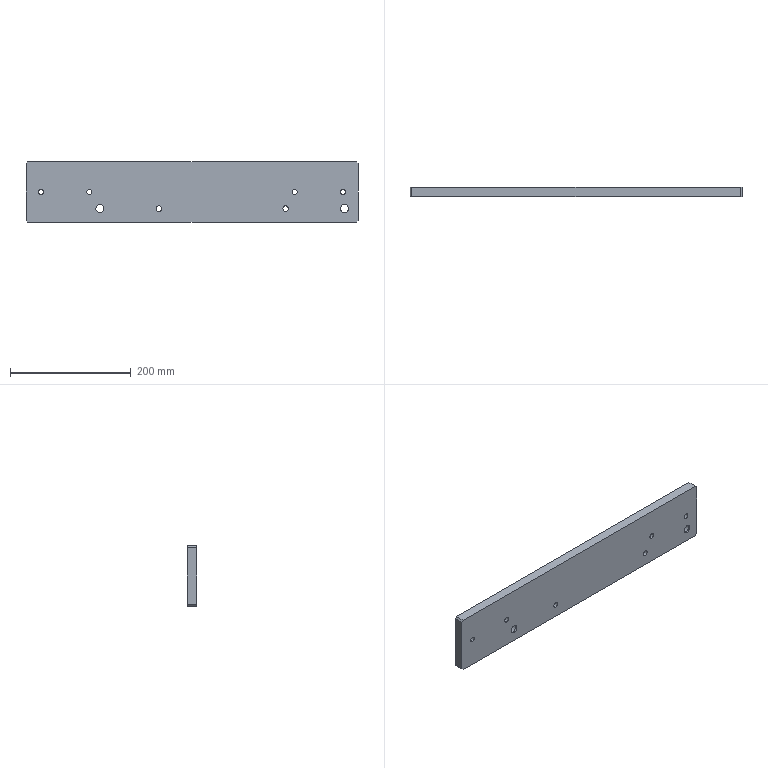Part | STEP file | PN_0058 | 1 solid | 38 faces | box 550 x 15 x 100 mm | volume 808868 mm3 | cylinder 24 | plane 14 | commonest cylinder face diameters 8.5 x8 9 x4 13.5 x4 15 x4 20 x4